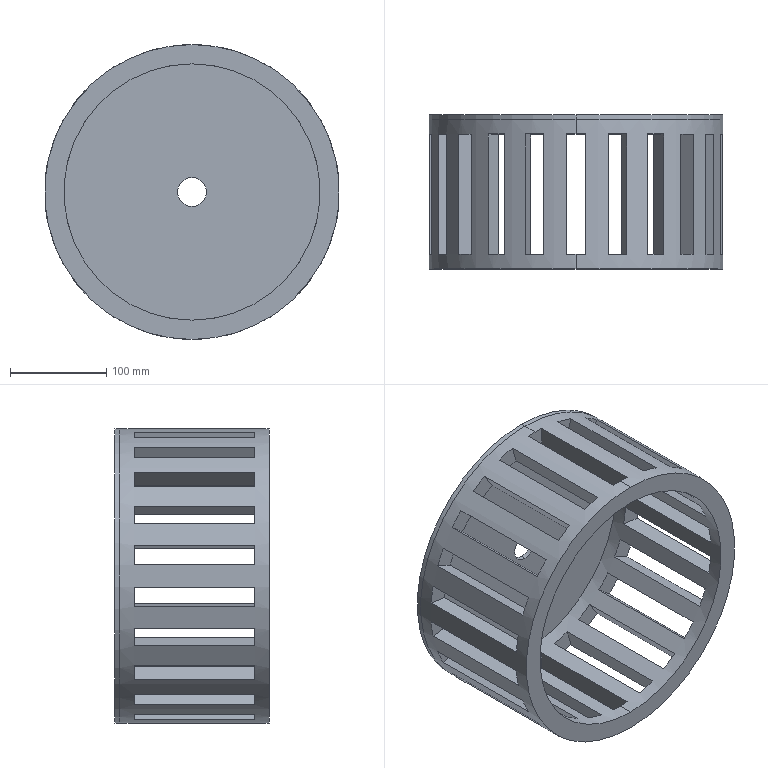Part | SolidWorks | features ICE 3, CirPattern 1, Extrusion 1 | 2 solids | 100 faces | box 306 x 160 x 306 mm | volume 2048607 mm3 | plane 92 | cylinder 8 | commonest cylinder face diameters 306 x4 30 x2 266 x2